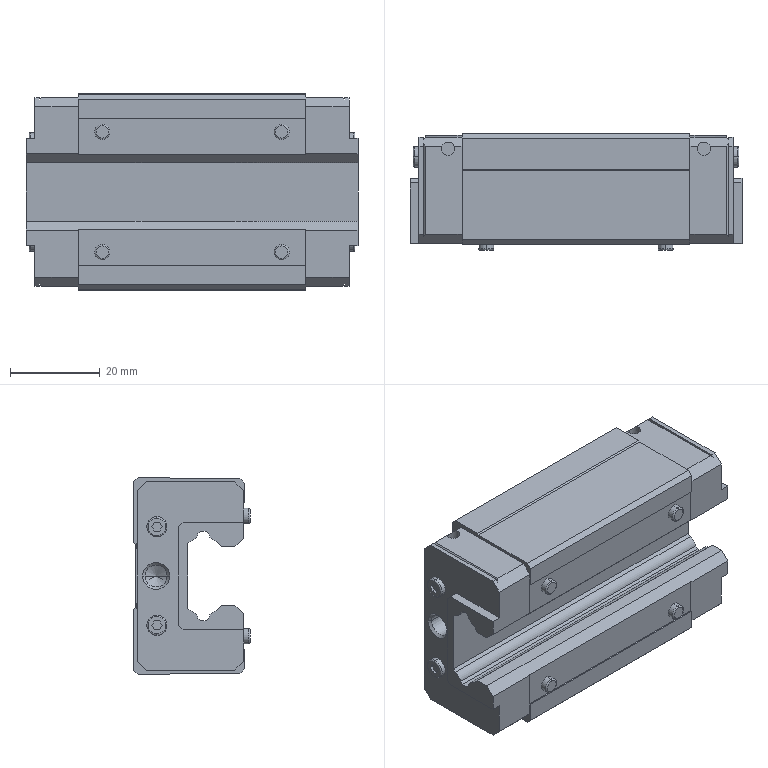Part | SolidWorks | features BaseBody 1 | 1 solid | 244 faces | box 74 x 26 x 44 mm | volume 58956 mm3 | plane 144 | cylinder 60 | cone 24 | torus 16 | commonest cylinder face diameters 4.134 x16 3 x8 3.43 x8 4.5 x8 4.917 x8 4.12 x4